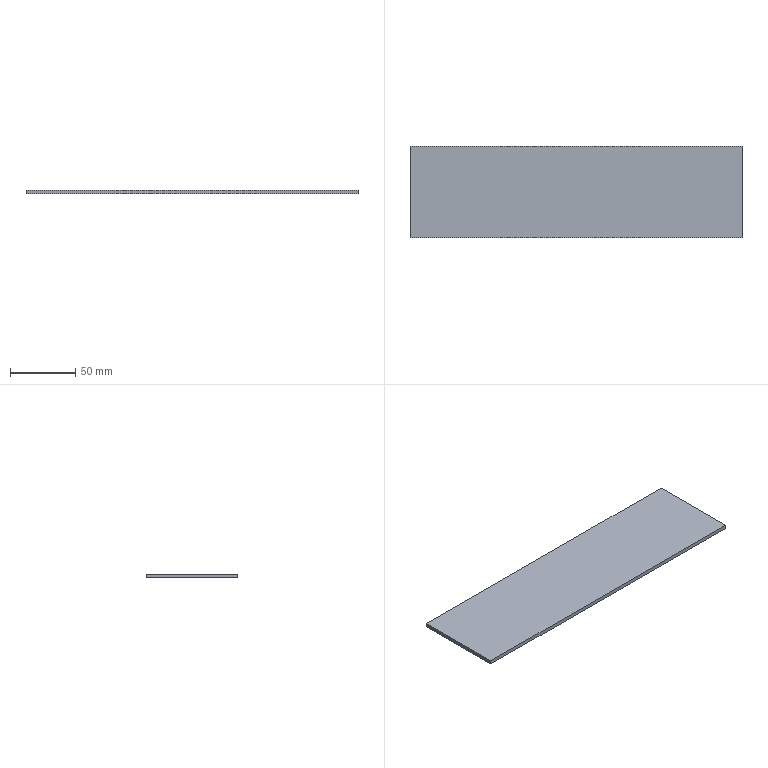Part | SolidWorks | features Extrusion 1 | 1 solid | 6 faces | box 255 x 70 x 3 mm | volume 53550 mm3 | plane 6
STEP:
#1=CARTESIAN_POINT('',(0.,70.,0.));
#2=VERTEX_POINT('',#1);
#3=CARTESIAN_POINT('',(0.,0.,0.));
#4=VERTEX_POINT('',#3);
#5=CARTESIAN_POINT('',(0.,70.,0.));
#6=DIRECTION('',(0.,-1.,0.));
#7=VECTOR('',#6,1000.);
#8=LINE('',#5,#7);
#9=EDGE_CURVE('',#2,#4,#8,.T.);
#10=ORIENTED_EDGE('',*,*,#9,.T.);
#11=CARTESIAN_POINT('',(0.,0.,3.));
#12=VERTEX_POINT('',#11);
#13=CARTESIAN_POINT('',(0.,0.,3.));
#14=DIRECTION('',(0.,0.,-1.));
#15=VECTOR('',#14,1000.);
#16=LINE('',#13,#15);
#17=EDGE_CURVE('',#12,#4,#16,.T.);
#18=ORIENTED_EDGE('',*,*,#17,.F.);
#19=CARTESIAN_POINT('',(0.,70.,3.));
#20=VERTEX_POINT('',#19);
#21=CARTESIAN_POINT('',(0.,70.,3.));
#22=DIRECTION('',(0.,-1.,0.));
#23=VECTOR('',#22,1000.);
#24=LINE('',#21,#23);
#25=EDGE_CURVE('',#20,#12,#24,.T.);
#26=ORIENTED_EDGE('',*,*,#25,.F.);
#27=CARTESIAN_POINT('',(0.,70.,3.));
#28=DIRECTION('',(0.,0.,-1.));
#29=VECTOR('',#28,1000.);
#30=LINE('',#27,#29);
#31=EDGE_CURVE('',#20,#2,#30,.T.);
#32=ORIENTED_EDGE('',*,*,#31,.T.);
#33=EDGE_LOOP('',(#10,#18,#26,#32));
#34=FACE_OUTER_BOUND('',#33,.T.);
#35=CARTESIAN_POINT('',(0.,70.,3.));
#36=DIRECTION('',(1.,0.,0.));
#37=DIRECTION('',(0.,0.,-1.));
#38=AXIS2_PLACEMENT_3D('',#35,#36,#37);
#39=PLANE('',#38);
#40=ADVANCED_FACE('',(#34),#39,.F.);
#41=CARTESIAN_POINT('',(255.,0.,0.));
#42=VERTEX_POINT('',#41);
#43=CARTESIAN_POINT('',(0.,0.,0.));
#44=DIRECTION('',(1.,0.,0.));
#45=VECTOR('',#44,1000.);
#46=LINE('',#43,#45);
#47=EDGE_CURVE('',#4,#42,#46,.T.);
#48=ORIENTED_EDGE('',*,*,#47,.T.);
#49=CARTESIAN_POINT('',(255.,0.,3.));
#50=VERTEX_POINT('',#49);
#51=CARTESIAN_POINT('',(255.,0.,3.));
#52=DIRECTION('',(0.,0.,-1.));
#53=VECTOR('',#52,1000.);
#54=LINE('',#51,#53);
#55=EDGE_CURVE('',#50,#42,#54,.T.);
#56=ORIENTED_EDGE('',*,*,#55,.F.);
#57=CARTESIAN_POINT('',(0.,0.,3.));
#58=DIRECTION('',(1.,0.,0.));
#59=VECTOR('',#58,1000.);
#60=LINE('',#57,#59);
#61=EDGE_CURVE('',#12,#50,#60,.T.);
#62=ORIENTED_EDGE('',*,*,#61,.F.);
#63=ORIENTED_EDGE('',*,*,#17,.T.);
#64=EDGE_LOOP('',(#48,#56,#62,#63));
#65=FACE_OUTER_BOUND('',#64,.T.);
#66=CARTESIAN_POINT('',(0.,0.,3.));
#67=DIRECTION('',(0.,1.,0.));
#68=DIRECTION('',(0.,0.,1.));
#69=AXIS2_PLACEMENT_3D('',#66,#67,#68);
#70=PLANE('',#69);
#71=ADVANCED_FACE('',(#65),#70,.F.);
#72=CARTESIAN_POINT('',(255.,70.,0.));
#73=VERTEX_POINT('',#72);
#74=CARTESIAN_POINT('',(255.,0.,0.));
#75=DIRECTION('',(0.,1.,0.));
#76=VECTOR('',#75,1000.);
#77=LINE('',#74,#76);
#78=EDGE_CURVE('',#42,#73,#77,.T.);
#79=ORIENTED_EDGE('',*,*,#78,.T.);
#80=CARTESIAN_POINT('',(255.,70.,3.));
#81=VERTEX_POINT('',#80);
#82=CARTESIAN_POINT('',(255.,70.,3.));
#83=DIRECTION('',(0.,0.,-1.));
#84=VECTOR('',#83,1000.);
#85=LINE('',#82,#84);
#86=EDGE_CURVE('',#81,#73,#85,.T.);
#87=ORIENTED_EDGE('',*,*,#86,.F.);
#88=CARTESIAN_POINT('',(255.,0.,3.));
#89=DIRECTION('',(0.,1.,0.));
#90=VECTOR('',#89,1000.);
#91=LINE('',#88,#90);
#92=EDGE_CURVE('',#50,#81,#91,.T.);
#93=ORIENTED_EDGE('',*,*,#92,.F.);
#94=ORIENTED_EDGE('',*,*,#55,.T.);
#95=EDGE_LOOP('',(#79,#87,#93,#94));
#96=FACE_OUTER_BOUND('',#95,.T.);
#97=CARTESIAN_POINT('',(255.,0.,3.));
#98=DIRECTION('',(-1.,0.,0.));
#99=DIRECTION('',(0.,0.,1.));
#100=AXIS2_PLACEMENT_3D('',#97,#98,#99);
#101=PLANE('',#100);
#102=ADVANCED_FACE('',(#96),#101,.F.);
#103=CARTESIAN_POINT('',(255.,70.,0.));
#104=DIRECTION('',(-1.,0.,0.));
#105=VECTOR('',#104,1000.);
#106=LINE('',#103,#105);
#107=EDGE_CURVE('',#73,#2,#106,.T.);
#108=ORIENTED_EDGE('',*,*,#107,.T.);
#109=ORIENTED_EDGE('',*,*,#31,.F.);
#110=CARTESIAN_POINT('',(255.,70.,3.));
#111=DIRECTION('',(-1.,0.,0.));
#112=VECTOR('',#111,1000.);
#113=LINE('',#110,#112);
#114=EDGE_CURVE('',#81,#20,#113,.T.);
#115=ORIENTED_EDGE('',*,*,#114,.F.);
#116=ORIENTED_EDGE('',*,*,#86,.T.);
#117=EDGE_LOOP('',(#108,#109,#115,#116));
#118=FACE_OUTER_BOUND('',#117,.T.);
#119=CARTESIAN_POINT('',(255.,70.,3.));
#120=DIRECTION('',(0.,-1.,0.));
#121=DIRECTION('',(0.,0.,-1.));
#122=AXIS2_PLACEMENT_3D('',#119,#120,#121);
#123=PLANE('',#122);
#124=ADVANCED_FACE('',(#118),#123,.F.);
#125=ORIENTED_EDGE('',*,*,#25,.T.);
#126=ORIENTED_EDGE('',*,*,#61,.T.);
#127=ORIENTED_EDGE('',*,*,#92,.T.);
#128=ORIENTED_EDGE('',*,*,#114,.T.);
#129=EDGE_LOOP('',(#125,#126,#127,#128));
#130=FACE_OUTER_BOUND('',#129,.T.);
#131=CARTESIAN_POINT('',(0.,0.,3.));
#132=DIRECTION('',(0.,0.,1.));
#133=DIRECTION('',(1.,0.,0.));
#134=AXIS2_PLACEMENT_3D('',#131,#132,#133);
#135=PLANE('',#134);
#136=ADVANCED_FACE('',(#130),#135,.T.);
#137=ORIENTED_EDGE('',*,*,#9,.F.);
#138=ORIENTED_EDGE('',*,*,#107,.F.);
#139=ORIENTED_EDGE('',*,*,#78,.F.);
#140=ORIENTED_EDGE('',*,*,#47,.F.);
#141=EDGE_LOOP('',(#137,#138,#139,#140));
#142=FACE_OUTER_BOUND('',#141,.T.);
#143=CARTESIAN_POINT('',(0.,0.,0.));
#144=DIRECTION('',(0.,0.,1.));
#145=DIRECTION('',(1.,0.,0.));
#146=AXIS2_PLACEMENT_3D('',#143,#144,#145);
#147=PLANE('',#146);
#148=ADVANCED_FACE('',(#142),#147,.F.);
#149=CLOSED_SHELL('',(#40,#71,#102,#124,#136,#148));
#150=MANIFOLD_SOLID_BREP('',#149);
#151=CARTESIAN_POINT('',(0.,0.,0.));
#152=DIRECTION('',(0.,0.,1.));
#153=DIRECTION('',(1.,0.,0.));
#154=AXIS2_PLACEMENT_3D('',#151,#152,#153);
#155=(LENGTH_UNIT()NAMED_UNIT(*)SI_UNIT(.MILLI.,.METRE.));
#156=UNCERTAINTY_MEASURE_WITH_UNIT(LENGTH_MEASURE(0.00001),#155,'','');
#157=(NAMED_UNIT(*)PLANE_ANGLE_UNIT()SI_UNIT($,.RADIAN.));
#158=(NAMED_UNIT(*)SI_UNIT($,.STERADIAN.)SOLID_ANGLE_UNIT());
#159=(GEOMETRIC_REPRESENTATION_CONTEXT(3)GLOBAL_UNCERTAINTY_ASSIGNED_CONTEXT((#156))GLOBAL_UNIT_ASSIGNED_CONTEXT((#155,#157,#158))REPRESENTATION_CONTEXT('',''));
#160=ADVANCED_BREP_SHAPE_REPRESENTATION('',(#150,#154),#159);